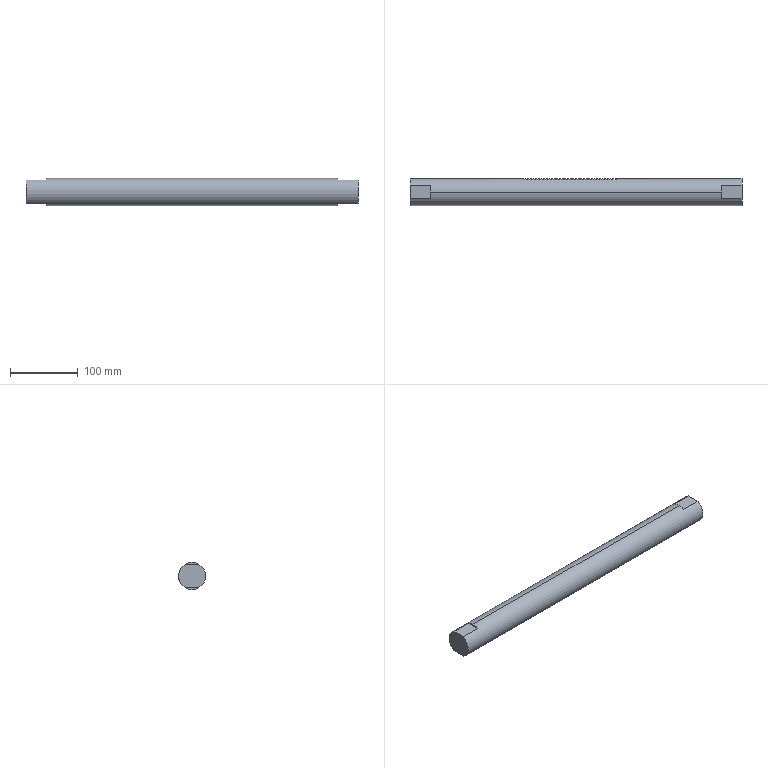Part | STEP file | Spur rack M1.25 length 160 | 1 solid | 119 faces | box 490 x 40 x 40 mm | volume 609575 mm3 | plane 117 | cylinder 2 | commonest cylinder face diameters 40 x2